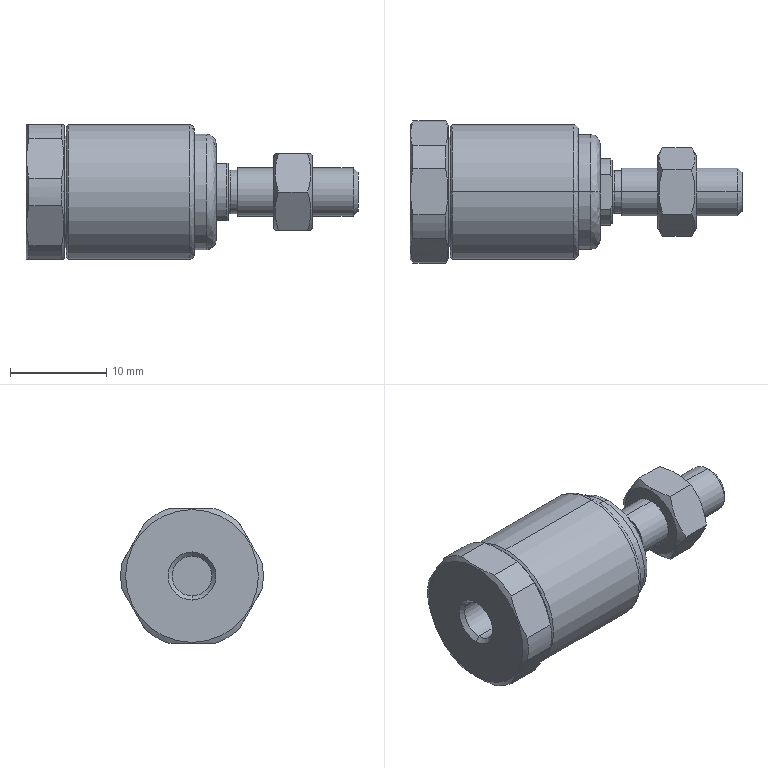Part | SolidWorks | features BaseBody 1 | 1 solid | 75 faces | box 34.5 x 14.8 x 14 mm | volume 3294 mm3 | plane 27 | cylinder 22 | cone 18 | spline 8 | commonest cylinder face diameters 14.8 x6 5 x4 4.134 x2 4.5 x2 7 x2 11.6 x2